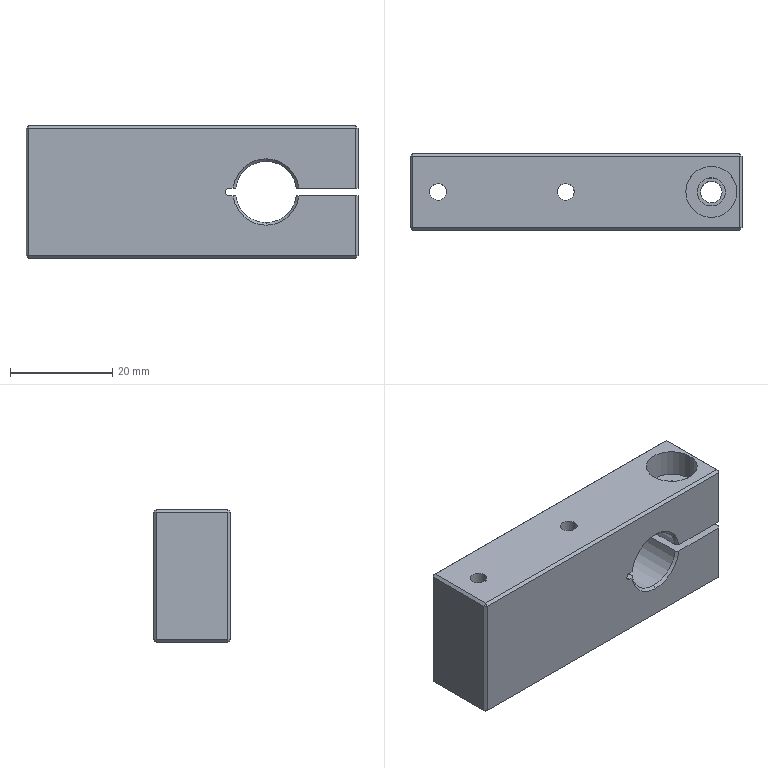Part | STEP file | ND25021-01-JDKM-32-TL | 1 solid | 55 faces | box 65 x 15 x 26 mm | volume 22080 mm3 | plane 34 | cylinder 15 | cone 6 | commonest cylinder face diameters 3.3 x4 12 x3 1.5 x2 4.2 x2 5.5 x2 10 x2